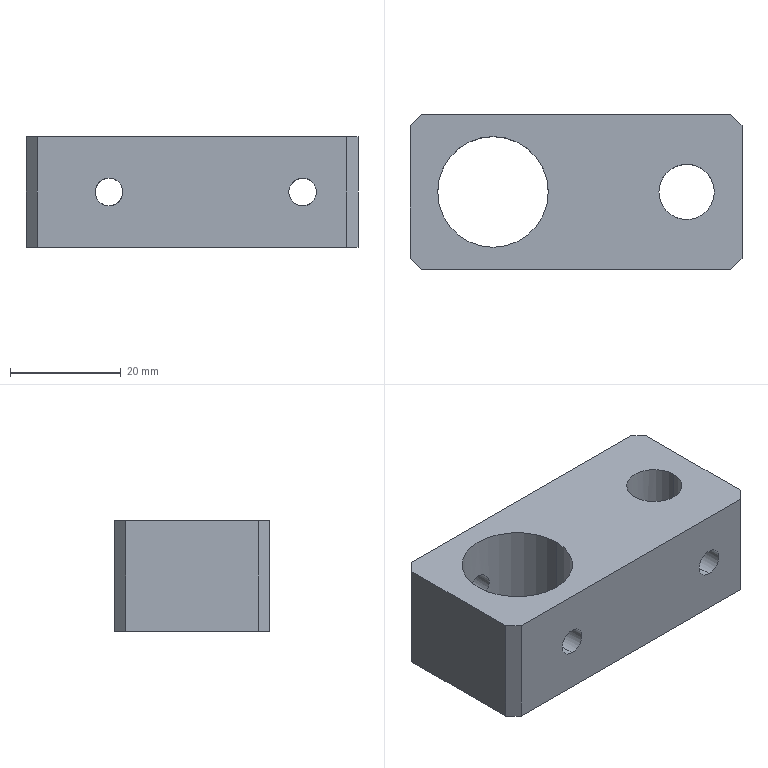Part | STEP file | Switch fixing block 1 | 1 solid | 22 faces | box 60 x 28 x 20 mm | volume 25066 mm3 | cylinder 12 | plane 10 | commonest cylinder face diameters 5 x8 10 x2 20 x2